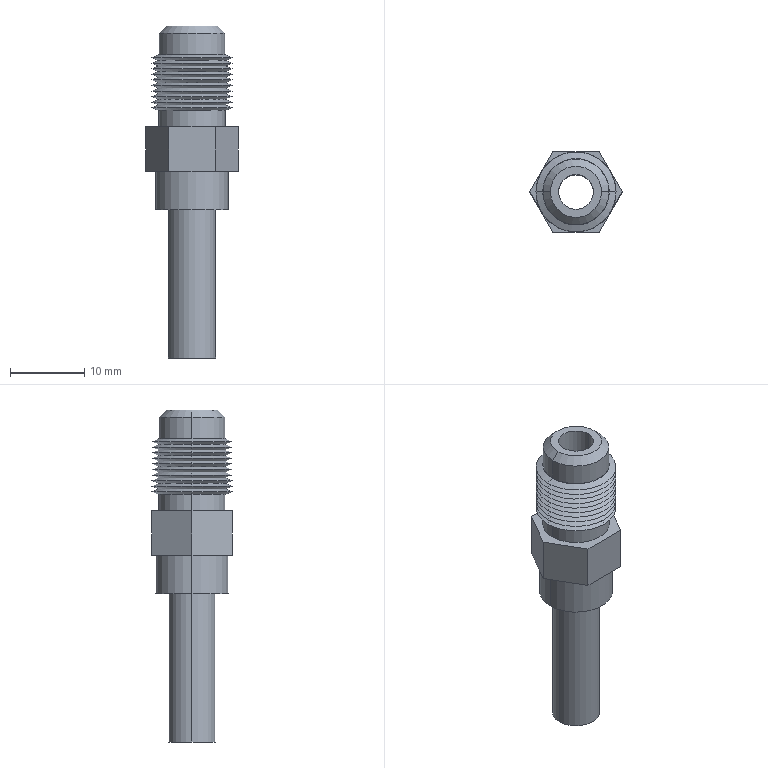Part | STEP file | liquid charging valve head | 12 solids | 108 faces | box 12.471 x 10.8 x 44.796 mm | volume 1804 mm3 | cone 43 | plane 33 | cylinder 32 | commonest cylinder face diameters 4.7 x24 6.35 x2 8.9 x2 9 x2 9.85 x2